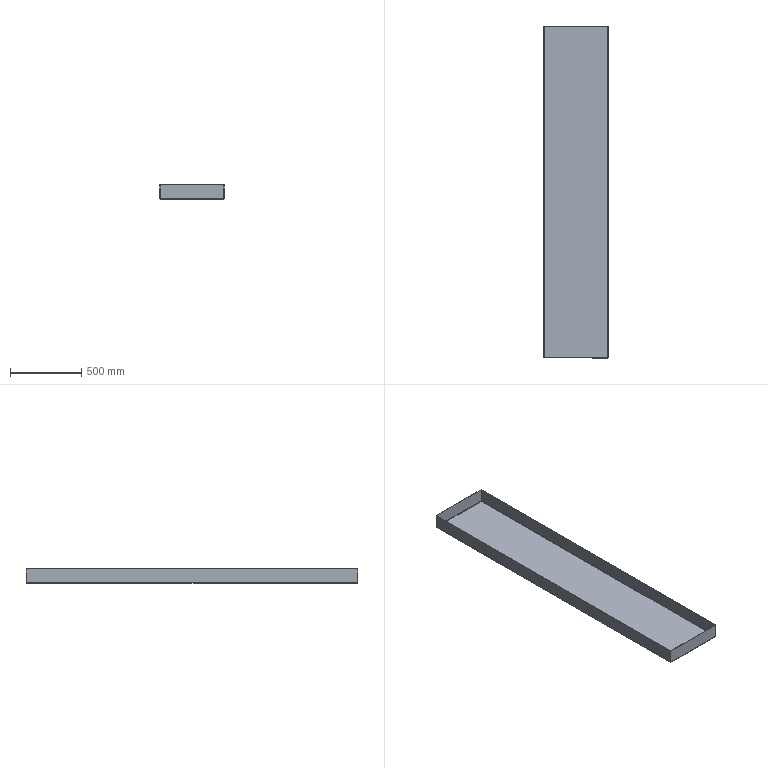Part | STEP file | 750038433 | 1 solid | 38 faces | box 450 x 2327 x 100 mm | volume 3164012 mm3 | plane 30 | cylinder 8 | commonest cylinder face diameters 4 x4 8 x4
STEP:
#1=CARTESIAN_POINT('',(-221.,2318.5,0.));
#2=VERTEX_POINT('',#1);
#3=CARTESIAN_POINT('',(221.,2318.5,0.));
#4=VERTEX_POINT('',#3);
#5=CARTESIAN_POINT('',(0.,2318.5,0.));
#6=DIRECTION('',(1.,0.,0.));
#7=VECTOR('',#6,1000.);
#8=LINE('',#5,#7);
#9=EDGE_CURVE('',#2,#4,#8,.T.);
#10=ORIENTED_EDGE('',*,*,#9,.T.);
#11=CARTESIAN_POINT('',(221.,0.,0.));
#12=VERTEX_POINT('',#11);
#13=CARTESIAN_POINT('',(221.,0.,0.));
#14=DIRECTION('',(0.,-1.,0.));
#15=VECTOR('',#14,1000.);
#16=LINE('',#13,#15);
#17=EDGE_CURVE('',#4,#12,#16,.T.);
#18=ORIENTED_EDGE('',*,*,#17,.T.);
#19=CARTESIAN_POINT('',(-221.,0.,0.));
#20=VERTEX_POINT('',#19);
#21=CARTESIAN_POINT('',(0.,0.,0.));
#22=DIRECTION('',(-1.,0.,0.));
#23=VECTOR('',#22,1000.);
#24=LINE('',#21,#23);
#25=EDGE_CURVE('',#12,#20,#24,.T.);
#26=ORIENTED_EDGE('',*,*,#25,.T.);
#27=CARTESIAN_POINT('',(-221.,0.,0.));
#28=DIRECTION('',(0.,1.,0.));
#29=VECTOR('',#28,1000.);
#30=LINE('',#27,#29);
#31=EDGE_CURVE('',#20,#2,#30,.T.);
#32=ORIENTED_EDGE('',*,*,#31,.T.);
#33=EDGE_LOOP('',(#10,#18,#26,#32));
#34=FACE_OUTER_BOUND('',#33,.T.);
#35=CARTESIAN_POINT('',(0.,0.,0.));
#36=DIRECTION('',(0.,0.,-1.));
#37=DIRECTION('',(-1.,0.,0.));
#38=AXIS2_PLACEMENT_3D('',#35,#36,#37);
#39=PLANE('',#38);
#40=ADVANCED_FACE('',(#34),#39,.T.);
#41=CARTESIAN_POINT('',(223.,2320.,0.5359));
#42=VERTEX_POINT('',#41);
#43=CARTESIAN_POINT('',(225.,2320.,4.));
#44=VERTEX_POINT('',#43);
#45=CARTESIAN_POINT('',(221.,2320.,4.));
#46=DIRECTION('',(0.,-1.,0.));
#47=DIRECTION('',(0.,0.,1.));
#48=AXIS2_PLACEMENT_3D('',#45,#46,#47);
#49=CIRCLE('',#48,4.);
#50=EDGE_CURVE('',#42,#44,#49,.T.);
#51=ORIENTED_EDGE('',*,*,#50,.T.);
#52=CARTESIAN_POINT('',(225.,-1.5,4.));
#53=VERTEX_POINT('',#52);
#54=CARTESIAN_POINT('',(225.,0.,4.));
#55=DIRECTION('',(0.,-1.,0.));
#56=VECTOR('',#55,1000.);
#57=LINE('',#54,#56);
#58=EDGE_CURVE('',#44,#53,#57,.T.);
#59=ORIENTED_EDGE('',*,*,#58,.T.);
#60=CARTESIAN_POINT('',(223.,-1.5,0.5359));
#61=VERTEX_POINT('',#60);
#62=CARTESIAN_POINT('',(221.,-1.5,4.));
#63=DIRECTION('',(0.,1.,0.));
#64=DIRECTION('',(0.,0.,1.));
#65=AXIS2_PLACEMENT_3D('',#62,#63,#64);
#66=CIRCLE('',#65,4.);
#67=EDGE_CURVE('',#53,#61,#66,.T.);
#68=ORIENTED_EDGE('',*,*,#67,.T.);
#69=CARTESIAN_POINT('',(223.,-1.5,0.5359));
#70=CARTESIAN_POINT('',(222.388,-1.041,0.1828));
#71=CARTESIAN_POINT('',(221.706,-0.5297,0.));
#72=CARTESIAN_POINT('',(221.,0.,0.));
#73=(BOUNDED_CURVE()B_SPLINE_CURVE(3,(#69,#70,#71,#72),.UNSPECIFIED.,.F.,.T.)B_SPLINE_CURVE_WITH_KNOTS((4,4),(4.189,4.712),.UNSPECIFIED.)CURVE()GEOMETRIC_REPRESENTATION_ITEM()RATIONAL_B_SPLINE_CURVE((1.,0.9773,0.9773,1.))REPRESENTATION_ITEM(''));
#74=EDGE_CURVE('',#61,#12,#73,.T.);
#75=ORIENTED_EDGE('',*,*,#74,.T.);
#76=ORIENTED_EDGE('',*,*,#17,.F.);
#77=CARTESIAN_POINT('',(221.,2318.5,0.));
#78=CARTESIAN_POINT('',(221.706,2319.03,0.));
#79=CARTESIAN_POINT('',(222.388,2319.541,0.1828));
#80=CARTESIAN_POINT('',(223.,2320.,0.5359));
#81=(BOUNDED_CURVE()B_SPLINE_CURVE(3,(#77,#78,#79,#80),.UNSPECIFIED.,.F.,.F.)B_SPLINE_CURVE_WITH_KNOTS((4,4),(4.712,5.236),.UNSPECIFIED.)CURVE()GEOMETRIC_REPRESENTATION_ITEM()RATIONAL_B_SPLINE_CURVE((1.,0.9773,0.9773,1.))REPRESENTATION_ITEM(''));
#82=EDGE_CURVE('',#4,#42,#81,.T.);
#83=ORIENTED_EDGE('',*,*,#82,.T.);
#84=EDGE_LOOP('',(#51,#59,#68,#75,#76,#83));
#85=FACE_OUTER_BOUND('',#84,.T.);
#86=CARTESIAN_POINT('',(221.,0.,4.));
#87=DIRECTION('',(0.,1.,0.));
#88=DIRECTION('',(0.,0.,1.));
#89=AXIS2_PLACEMENT_3D('',#86,#87,#88);
#90=CYLINDRICAL_SURFACE('',#89,4.);
#91=ADVANCED_FACE('',(#85),#90,.T.);
#92=CARTESIAN_POINT('',(222.5,2320.5,0.5359));
#93=VERTEX_POINT('',#92);
#94=CARTESIAN_POINT('',(222.5,2320.5,0.5359));
#95=CARTESIAN_POINT('',(222.041,2319.888,0.1828));
#96=CARTESIAN_POINT('',(221.53,2319.206,0.));
#97=CARTESIAN_POINT('',(221.,2318.5,0.));
#98=(BOUNDED_CURVE()B_SPLINE_CURVE(3,(#94,#95,#96,#97),.UNSPECIFIED.,.F.,.F.)B_SPLINE_CURVE_WITH_KNOTS((4,4),(4.189,4.712),.UNSPECIFIED.)CURVE()GEOMETRIC_REPRESENTATION_ITEM()RATIONAL_B_SPLINE_CURVE((1.,0.9773,0.9773,1.))REPRESENTATION_ITEM(''));
#99=EDGE_CURVE('',#93,#4,#98,.T.);
#100=ORIENTED_EDGE('',*,*,#99,.T.);
#101=ORIENTED_EDGE('',*,*,#9,.F.);
#102=CARTESIAN_POINT('',(-222.5,2320.5,0.5359));
#103=VERTEX_POINT('',#102);
#104=CARTESIAN_POINT('',(-221.,2318.5,0.));
#105=CARTESIAN_POINT('',(-221.53,2319.206,0.));
#106=CARTESIAN_POINT('',(-222.041,2319.888,0.1828));
#107=CARTESIAN_POINT('',(-222.5,2320.5,0.5359));
#108=(BOUNDED_CURVE()B_SPLINE_CURVE(3,(#104,#105,#106,#107),.UNSPECIFIED.,.F.,.T.)B_SPLINE_CURVE_WITH_KNOTS((4,4),(4.712,5.236),.UNSPECIFIED.)CURVE()GEOMETRIC_REPRESENTATION_ITEM()RATIONAL_B_SPLINE_CURVE((1.,0.9773,0.9773,1.))REPRESENTATION_ITEM(''));
#109=EDGE_CURVE('',#2,#103,#108,.T.);
#110=ORIENTED_EDGE('',*,*,#109,.T.);
#111=CARTESIAN_POINT('',(-222.5,2322.5,4.));
#112=VERTEX_POINT('',#111);
#113=CARTESIAN_POINT('',(-222.5,2318.5,4.));
#114=DIRECTION('',(1.,0.,0.));
#115=DIRECTION('',(0.,-1.,0.));
#116=AXIS2_PLACEMENT_3D('',#113,#114,#115);
#117=CIRCLE('',#116,4.);
#118=EDGE_CURVE('',#103,#112,#117,.T.);
#119=ORIENTED_EDGE('',*,*,#118,.T.);
#120=CARTESIAN_POINT('',(222.5,2322.5,4.));
#121=VERTEX_POINT('',#120);
#122=CARTESIAN_POINT('',(221.,2322.5,4.));
#123=DIRECTION('',(1.,0.,0.));
#124=VECTOR('',#123,1000.);
#125=LINE('',#122,#124);
#126=EDGE_CURVE('',#112,#121,#125,.T.);
#127=ORIENTED_EDGE('',*,*,#126,.T.);
#128=CARTESIAN_POINT('',(222.5,2318.5,4.));
#129=DIRECTION('',(-1.,0.,0.));
#130=DIRECTION('',(0.,-1.,0.));
#131=AXIS2_PLACEMENT_3D('',#128,#129,#130);
#132=CIRCLE('',#131,4.);
#133=EDGE_CURVE('',#121,#93,#132,.T.);
#134=ORIENTED_EDGE('',*,*,#133,.T.);
#135=EDGE_LOOP('',(#100,#101,#110,#119,#127,#134));
#136=FACE_OUTER_BOUND('',#135,.T.);
#137=CARTESIAN_POINT('',(221.,2318.5,4.));
#138=DIRECTION('',(-1.,0.,0.));
#139=DIRECTION('',(0.,-1.,0.));
#140=AXIS2_PLACEMENT_3D('',#137,#138,#139);
#141=CYLINDRICAL_SURFACE('',#140,4.);
#142=ADVANCED_FACE('',(#136),#141,.T.);
#143=CARTESIAN_POINT('',(-223.,2320.,0.5359));
#144=VERTEX_POINT('',#143);
#145=CARTESIAN_POINT('',(-223.,2320.,0.5359));
#146=CARTESIAN_POINT('',(-222.388,2319.541,0.1828));
#147=CARTESIAN_POINT('',(-221.706,2319.03,0.));
#148=CARTESIAN_POINT('',(-221.,2318.5,0.));
#149=(BOUNDED_CURVE()B_SPLINE_CURVE(3,(#145,#146,#147,#148),.UNSPECIFIED.,.F.,.F.)B_SPLINE_CURVE_WITH_KNOTS((4,4),(4.189,4.712),.UNSPECIFIED.)CURVE()GEOMETRIC_REPRESENTATION_ITEM()RATIONAL_B_SPLINE_CURVE((1.,0.9773,0.9773,1.))REPRESENTATION_ITEM(''));
#150=EDGE_CURVE('',#144,#2,#149,.T.);
#151=ORIENTED_EDGE('',*,*,#150,.T.);
#152=ORIENTED_EDGE('',*,*,#31,.F.);
#153=CARTESIAN_POINT('',(-223.,-1.5,0.5359));
#154=VERTEX_POINT('',#153);
#155=CARTESIAN_POINT('',(-221.,0.,0.));
#156=CARTESIAN_POINT('',(-221.706,-0.5297,0.));
#157=CARTESIAN_POINT('',(-222.388,-1.041,0.1828));
#158=CARTESIAN_POINT('',(-223.,-1.5,0.5359));
#159=(BOUNDED_CURVE()B_SPLINE_CURVE(3,(#155,#156,#157,#158),.UNSPECIFIED.,.F.,.T.)B_SPLINE_CURVE_WITH_KNOTS((4,4),(4.712,5.236),.UNSPECIFIED.)CURVE()GEOMETRIC_REPRESENTATION_ITEM()RATIONAL_B_SPLINE_CURVE((1.,0.9773,0.9773,1.))REPRESENTATION_ITEM(''));
#160=EDGE_CURVE('',#20,#154,#159,.T.);
#161=ORIENTED_EDGE('',*,*,#160,.T.);
#162=CARTESIAN_POINT('',(-225.,-1.5,4.));
#163=VERTEX_POINT('',#162);
#164=CARTESIAN_POINT('',(-221.,-1.5,4.));
#165=DIRECTION('',(0.,1.,0.));
#166=DIRECTION('',(0.,0.,-1.));
#167=AXIS2_PLACEMENT_3D('',#164,#165,#166);
#168=CIRCLE('',#167,4.);
#169=EDGE_CURVE('',#154,#163,#168,.T.);
#170=ORIENTED_EDGE('',*,*,#169,.T.);
#171=CARTESIAN_POINT('',(-225.,2320.,4.));
#172=VERTEX_POINT('',#171);
#173=CARTESIAN_POINT('',(-225.,2318.5,4.));
#174=DIRECTION('',(0.,1.,0.));
#175=VECTOR('',#174,1000.);
#176=LINE('',#173,#175);
#177=EDGE_CURVE('',#163,#172,#176,.T.);
#178=ORIENTED_EDGE('',*,*,#177,.T.);
#179=CARTESIAN_POINT('',(-221.,2320.,4.));
#180=DIRECTION('',(0.,-1.,0.));
#181=DIRECTION('',(0.,0.,-1.));
#182=AXIS2_PLACEMENT_3D('',#179,#180,#181);
#183=CIRCLE('',#182,4.);
#184=EDGE_CURVE('',#172,#144,#183,.T.);
#185=ORIENTED_EDGE('',*,*,#184,.T.);
#186=EDGE_LOOP('',(#151,#152,#161,#170,#178,#185));
#187=FACE_OUTER_BOUND('',#186,.T.);
#188=CARTESIAN_POINT('',(-221.,2318.5,4.));
#189=DIRECTION('',(0.,-1.,0.));
#190=DIRECTION('',(0.,0.,-1.));
#191=AXIS2_PLACEMENT_3D('',#188,#189,#190);
#192=CYLINDRICAL_SURFACE('',#191,4.);
#193=ADVANCED_FACE('',(#187),#192,.T.);
#194=CARTESIAN_POINT('',(-222.5,-2.,0.5359));
#195=VERTEX_POINT('',#194);
#196=CARTESIAN_POINT('',(-222.5,-2.,0.5359));
#197=CARTESIAN_POINT('',(-222.041,-1.388,0.1828));
#198=CARTESIAN_POINT('',(-221.53,-0.7062,0.));
#199=CARTESIAN_POINT('',(-221.,0.,0.));
#200=(BOUNDED_CURVE()B_SPLINE_CURVE(3,(#196,#197,#198,#199),.UNSPECIFIED.,.F.,.F.)B_SPLINE_CURVE_WITH_KNOTS((4,4),(4.189,4.712),.UNSPECIFIED.)CURVE()GEOMETRIC_REPRESENTATION_ITEM()RATIONAL_B_SPLINE_CURVE((1.,0.9773,0.9773,1.))REPRESENTATION_ITEM(''));
#201=EDGE_CURVE('',#195,#20,#200,.T.);
#202=ORIENTED_EDGE('',*,*,#201,.T.);
#203=ORIENTED_EDGE('',*,*,#25,.F.);
#204=CARTESIAN_POINT('',(222.5,-2.,0.5359));
#205=VERTEX_POINT('',#204);
#206=CARTESIAN_POINT('',(221.,0.,0.));
#207=CARTESIAN_POINT('',(221.53,-0.7062,0.));
#208=CARTESIAN_POINT('',(222.041,-1.388,0.1828));
#209=CARTESIAN_POINT('',(222.5,-2.,0.5359));
#210=(BOUNDED_CURVE()B_SPLINE_CURVE(3,(#206,#207,#208,#209),.UNSPECIFIED.,.F.,.F.)B_SPLINE_CURVE_WITH_KNOTS((4,4),(4.712,5.236),.UNSPECIFIED.)CURVE()GEOMETRIC_REPRESENTATION_ITEM()RATIONAL_B_SPLINE_CURVE((1.,0.9773,0.9773,1.))REPRESENTATION_ITEM(''));
#211=EDGE_CURVE('',#12,#205,#210,.T.);
#212=ORIENTED_EDGE('',*,*,#211,.T.);
#213=CARTESIAN_POINT('',(222.5,-4.,4.));
#214=VERTEX_POINT('',#213);
#215=CARTESIAN_POINT('',(222.5,0.,4.));
#216=DIRECTION('',(-1.,0.,0.));
#217=DIRECTION('',(0.,1.,0.));
#218=AXIS2_PLACEMENT_3D('',#215,#216,#217);
#219=CIRCLE('',#218,4.);
#220=EDGE_CURVE('',#205,#214,#219,.T.);
#221=ORIENTED_EDGE('',*,*,#220,.T.);
#222=CARTESIAN_POINT('',(-222.5,-4.,4.));
#223=VERTEX_POINT('',#222);
#224=CARTESIAN_POINT('',(-221.,-4.,4.));
#225=DIRECTION('',(-1.,0.,0.));
#226=VECTOR('',#225,1000.);
#227=LINE('',#224,#226);
#228=EDGE_CURVE('',#214,#223,#227,.T.);
#229=ORIENTED_EDGE('',*,*,#228,.T.);
#230=CARTESIAN_POINT('',(-222.5,0.,4.));
#231=DIRECTION('',(1.,0.,0.));
#232=DIRECTION('',(0.,1.,0.));
#233=AXIS2_PLACEMENT_3D('',#230,#231,#232);
#234=CIRCLE('',#233,4.);
#235=EDGE_CURVE('',#223,#195,#234,.T.);
#236=ORIENTED_EDGE('',*,*,#235,.T.);
#237=EDGE_LOOP('',(#202,#203,#212,#221,#229,#236));
#238=FACE_OUTER_BOUND('',#237,.T.);
#239=CARTESIAN_POINT('',(-221.,0.,4.));
#240=DIRECTION('',(1.,0.,0.));
#241=DIRECTION('',(0.,1.,0.));
#242=AXIS2_PLACEMENT_3D('',#239,#240,#241);
#243=CYLINDRICAL_SURFACE('',#242,4.);
#244=ADVANCED_FACE('',(#238),#243,.T.);
#245=CARTESIAN_POINT('',(225.,2320.,100.));
#246=VERTEX_POINT('',#245);
#247=CARTESIAN_POINT('',(225.,2320.,0.));
#248=DIRECTION('',(0.,0.,-1.));
#249=VECTOR('',#248,1000.);
#250=LINE('',#247,#249);
#251=EDGE_CURVE('',#246,#44,#250,.T.);
#252=ORIENTED_EDGE('',*,*,#251,.F.);
#253=CARTESIAN_POINT('',(225.,-1.5,100.));
#254=VERTEX_POINT('',#253);
#255=CARTESIAN_POINT('',(225.,0.,100.));
#256=DIRECTION('',(0.,1.,0.));
#257=VECTOR('',#256,1000.);
#258=LINE('',#255,#257);
#259=EDGE_CURVE('',#254,#246,#258,.T.);
#260=ORIENTED_EDGE('',*,*,#259,.F.);
#261=CARTESIAN_POINT('',(225.,-1.5,0.));
#262=DIRECTION('',(0.,0.,1.));
#263=VECTOR('',#262,1000.);
#264=LINE('',#261,#263);
#265=EDGE_CURVE('',#53,#254,#264,.T.);
#266=ORIENTED_EDGE('',*,*,#265,.F.);
#267=ORIENTED_EDGE('',*,*,#58,.F.);
#268=EDGE_LOOP('',(#252,#260,#266,#267));
#269=FACE_OUTER_BOUND('',#268,.T.);
#270=CARTESIAN_POINT('',(225.,0.,0.));
#271=DIRECTION('',(-1.,0.,0.));
#272=DIRECTION('',(0.,-1.,0.));
#273=AXIS2_PLACEMENT_3D('',#270,#271,#272);
#274=PLANE('',#273);
#275=ADVANCED_FACE('',(#269),#274,.F.);
#276=CARTESIAN_POINT('',(223.,2320.,4.));
#277=VERTEX_POINT('',#276);
#278=CARTESIAN_POINT('',(223.,2320.,100.));
#279=VERTEX_POINT('',#278);
#280=CARTESIAN_POINT('',(223.,2320.,2.));
#281=DIRECTION('',(0.,0.,1.));
#282=VECTOR('',#281,1000.);
#283=LINE('',#280,#282);
#284=EDGE_CURVE('',#277,#279,#283,.T.);
#285=ORIENTED_EDGE('',*,*,#284,.T.);
#286=CARTESIAN_POINT('',(-221.,2320.,100.));
#287=DIRECTION('',(1.,0.,0.));
#288=VECTOR('',#287,1000.);
#289=LINE('',#286,#288);
#290=EDGE_CURVE('',#279,#246,#289,.T.);
#291=ORIENTED_EDGE('',*,*,#290,.T.);
#292=ORIENTED_EDGE('',*,*,#251,.T.);
#293=ORIENTED_EDGE('',*,*,#50,.F.);
#294=CARTESIAN_POINT('',(223.,2320.,2.));
#295=DIRECTION('',(0.,0.,1.));
#296=VECTOR('',#295,1000.);
#297=LINE('',#294,#296);
#298=EDGE_CURVE('',#42,#277,#297,.T.);
#299=ORIENTED_EDGE('',*,*,#298,.T.);
#300=EDGE_LOOP('',(#285,#291,#292,#293,#299));
#301=FACE_OUTER_BOUND('',#300,.T.);
#302=CARTESIAN_POINT('',(-221.,2320.,2.));
#303=DIRECTION('',(0.,1.,0.));
#304=DIRECTION('',(0.,0.,1.));
#305=AXIS2_PLACEMENT_3D('',#302,#303,#304);
#306=PLANE('',#305);
#307=ADVANCED_FACE('',(#301),#306,.T.);
#308=ORIENTED_EDGE('',*,*,#298,.F.);
#309=ORIENTED_EDGE('',*,*,#82,.F.);
#310=CARTESIAN_POINT('',(221.,2318.5,2.));
#311=VERTEX_POINT('',#310);
#312=CARTESIAN_POINT('',(221.,2318.5,-1000.));
#313=DIRECTION('',(0.,0.,-1.));
#314=VECTOR('',#313,1000.);
#315=LINE('',#312,#314);
#316=EDGE_CURVE('',#311,#4,#315,.T.);
#317=ORIENTED_EDGE('',*,*,#316,.F.);
#318=CARTESIAN_POINT('',(223.,2320.,4.));
#319=CARTESIAN_POINT('',(223.,2320.,2.828));
#320=CARTESIAN_POINT('',(222.172,2319.379,2.));
#321=CARTESIAN_POINT('',(221.,2318.5,2.));
#322=(BOUNDED_CURVE()B_SPLINE_CURVE(3,(#318,#319,#320,#321),.UNSPECIFIED.,.F.,.F.)B_SPLINE_CURVE_WITH_KNOTS((4,4),(0.,1.571),.UNSPECIFIED.)CURVE()GEOMETRIC_REPRESENTATION_ITEM()RATIONAL_B_SPLINE_CURVE((1.,0.8047,0.8047,1.))REPRESENTATION_ITEM(''));
#323=EDGE_CURVE('',#277,#311,#322,.T.);
#324=ORIENTED_EDGE('',*,*,#323,.F.);
#325=EDGE_LOOP('',(#308,#309,#317,#324));
#326=FACE_OUTER_BOUND('',#325,.T.);
#327=CARTESIAN_POINT('',(-579.,1718.5,-1000.));
#328=DIRECTION('',(0.6,-0.8,0.));
#329=DIRECTION('',(0.8,0.6,0.));
#330=AXIS2_PLACEMENT_3D('',#327,#328,#329);
#331=PLANE('',#330);
#332=ADVANCED_FACE('',(#326),#331,.F.);
#333=CARTESIAN_POINT('',(221.,0.,2.));
#334=VERTEX_POINT('',#333);
#335=CARTESIAN_POINT('',(221.,0.,-1000.));
#336=DIRECTION('',(0.,0.,-1.));
#337=VECTOR('',#336,1000.);
#338=LINE('',#335,#337);
#339=EDGE_CURVE('',#334,#12,#338,.T.);
#340=ORIENTED_EDGE('',*,*,#339,.T.);
#341=ORIENTED_EDGE('',*,*,#74,.F.);
#342=CARTESIAN_POINT('',(223.,-1.5,4.));
#343=VERTEX_POINT('',#342);
#344=CARTESIAN_POINT('',(223.,-1.5,-1000.));
#345=DIRECTION('',(0.,0.,1.));
#346=VECTOR('',#345,1000.);
#347=LINE('',#344,#346);
#348=EDGE_CURVE('',#61,#343,#347,.T.);
#349=ORIENTED_EDGE('',*,*,#348,.T.);
#350=CARTESIAN_POINT('',(223.,-1.5,4.));
#351=CARTESIAN_POINT('',(223.,-1.5,2.828));
#352=CARTESIAN_POINT('',(222.172,-0.8787,2.));
#353=CARTESIAN_POINT('',(221.,0.,2.));
#354=(BOUNDED_CURVE()B_SPLINE_CURVE(3,(#350,#351,#352,#353),.UNSPECIFIED.,.F.,.F.)B_SPLINE_CURVE_WITH_KNOTS((4,4),(3.142,4.712),.UNSPECIFIED.)CURVE()GEOMETRIC_REPRESENTATION_ITEM()RATIONAL_B_SPLINE_CURVE((1.,0.8047,0.8047,1.))REPRESENTATION_ITEM(''));
#355=EDGE_CURVE('',#343,#334,#354,.T.);
#356=ORIENTED_EDGE('',*,*,#355,.T.);
#357=EDGE_LOOP('',(#340,#341,#349,#356));
#358=FACE_OUTER_BOUND('',#357,.T.);
#359=CARTESIAN_POINT('',(-579.,600.,-1000.));
#360=DIRECTION('',(-0.6,-0.8,0.));
#361=DIRECTION('',(0.8,-0.6,0.));
#362=AXIS2_PLACEMENT_3D('',#359,#360,#361);
#363=PLANE('',#362);
#364=ADVANCED_FACE('',(#358),#363,.T.);
#365=ORIENTED_EDGE('',*,*,#265,.T.);
#366=CARTESIAN_POINT('',(223.,-1.5,100.));
#367=VERTEX_POINT('',#366);
#368=CARTESIAN_POINT('',(221.,-1.5,100.));
#369=DIRECTION('',(-1.,0.,0.));
#370=VECTOR('',#369,1000.);
#371=LINE('',#368,#370);
#372=EDGE_CURVE('',#254,#367,#371,.T.);
#373=ORIENTED_EDGE('',*,*,#372,.T.);
#374=CARTESIAN_POINT('',(223.,-1.5,2.));
#375=DIRECTION('',(0.,0.,-1.));
#376=VECTOR('',#375,1000.);
#377=LINE('',#374,#376);
#378=EDGE_CURVE('',#367,#343,#377,.T.);
#379=ORIENTED_EDGE('',*,*,#378,.T.);
#380=ORIENTED_EDGE('',*,*,#348,.F.);
#381=ORIENTED_EDGE('',*,*,#67,.F.);
#382=EDGE_LOOP('',(#365,#373,#379,#380,#381));
#383=FACE_OUTER_BOUND('',#382,.T.);
#384=CARTESIAN_POINT('',(221.,-1.5,2.));
#385=DIRECTION('',(0.,-1.,0.));
#386=DIRECTION('',(0.,0.,-1.));
#387=AXIS2_PLACEMENT_3D('',#384,#385,#386);
#388=PLANE('',#387);
#389=ADVANCED_FACE('',(#383),#388,.T.);
#390=CARTESIAN_POINT('',(222.5,2320.5,4.));
#391=VERTEX_POINT('',#390);
#392=CARTESIAN_POINT('',(222.5,2320.5,4.));
#393=CARTESIAN_POINT('',(222.5,2320.5,2.828));
#394=CARTESIAN_POINT('',(221.879,2319.672,2.));
#395=CARTESIAN_POINT('',(221.,2318.5,2.));
#396=(BOUNDED_CURVE()B_SPLINE_CURVE(3,(#392,#393,#394,#395),.UNSPECIFIED.,.F.,.F.)B_SPLINE_CURVE_WITH_KNOTS((4,4),(3.142,4.712),.UNSPECIFIED.)CURVE()GEOMETRIC_REPRESENTATION_ITEM()RATIONAL_B_SPLINE_CURVE((1.,0.8047,0.8047,1.))REPRESENTATION_ITEM(''));
#397=EDGE_CURVE('',#391,#311,#396,.T.);
#398=ORIENTED_EDGE('',*,*,#397,.T.);
#399=ORIENTED_EDGE('',*,*,#316,.T.);
#400=ORIENTED_EDGE('',*,*,#99,.F.);
#401=CARTESIAN_POINT('',(222.5,2320.5,-1000.));
#402=DIRECTION('',(0.,0.,1.));
#403=VECTOR('',#402,1000.);
#404=LINE('',#401,#403);
#405=EDGE_CURVE('',#93,#391,#404,.T.);
#406=ORIENTED_EDGE('',*,*,#405,.T.);
#407=EDGE_LOOP('',(#398,#399,#400,#406));
#408=FACE_OUTER_BOUND('',#407,.T.);
#409=CARTESIAN_POINT('',(-379.,1518.5,-1000.));
#410=DIRECTION('',(0.8,-0.6,0.));
#411=DIRECTION('',(0.6,0.8,0.));
#412=AXIS2_PLACEMENT_3D('',#409,#410,#411);
#413=PLANE('',#412);
#414=ADVANCED_FACE('',(#408),#413,.T.);
#415=ORIENTED_EDGE('',*,*,#405,.F.);
#416=ORIENTED_EDGE('',*,*,#133,.F.);
#417=CARTESIAN_POINT('',(222.5,2322.5,100.));
#418=VERTEX_POINT('',#417);
#419=CARTESIAN_POINT('',(222.5,2322.5,100.));
#420=DIRECTION('',(0.,0.,-1.));
#421=VECTOR('',#420,1000.);
#422=LINE('',#419,#421);
#423=EDGE_CURVE('',#418,#121,#422,.T.);
#424=ORIENTED_EDGE('',*,*,#423,.F.);
#425=CARTESIAN_POINT('',(222.5,2320.5,100.));
#426=VERTEX_POINT('',#425);
#427=CARTESIAN_POINT('',(222.5,2322.5,100.));
#428=DIRECTION('',(0.,1.,0.));
#429=VECTOR('',#428,1000.);
#430=LINE('',#427,#429);
#431=EDGE_CURVE('',#426,#418,#430,.T.);
#432=ORIENTED_EDGE('',*,*,#431,.F.);
#433=CARTESIAN_POINT('',(222.5,2320.5,100.));
#434=DIRECTION('',(0.,0.,1.));
#435=VECTOR('',#434,1000.);
#436=LINE('',#433,#435);
#437=EDGE_CURVE('',#391,#426,#436,.T.);
#438=ORIENTED_EDGE('',*,*,#437,.F.);
#439=EDGE_LOOP('',(#415,#416,#424,#432,#438));
#440=FACE_OUTER_BOUND('',#439,.T.);
#441=CARTESIAN_POINT('',(222.5,2322.5,100.));
#442=DIRECTION('',(-1.,0.,0.));
#443=DIRECTION('',(0.,0.,1.));
#444=AXIS2_PLACEMENT_3D('',#441,#442,#443);
#445=PLANE('',#444);
#446=ADVANCED_FACE('',(#440),#445,.F.);
#447=CARTESIAN_POINT('',(-222.5,2322.5,100.));
#448=VERTEX_POINT('',#447);
#449=CARTESIAN_POINT('',(-222.5,2322.5,0.));
#450=DIRECTION('',(0.,0.,1.));
#451=VECTOR('',#450,1000.);
#452=LINE('',#449,#451);
#453=EDGE_CURVE('',#112,#448,#452,.T.);
#454=ORIENTED_EDGE('',*,*,#453,.T.);
#455=CARTESIAN_POINT('',(0.,2322.5,100.));
#456=DIRECTION('',(1.,0.,0.));
#457=VECTOR('',#456,1000.);
#458=LINE('',#455,#457);
#459=EDGE_CURVE('',#448,#418,#458,.T.);
#460=ORIENTED_EDGE('',*,*,#459,.T.);
#461=ORIENTED_EDGE('',*,*,#423,.T.);
#462=ORIENTED_EDGE('',*,*,#126,.F.);
#463=EDGE_LOOP('',(#454,#460,#461,#462));
#464=FACE_OUTER_BOUND('',#463,.T.);
#465=CARTESIAN_POINT('',(0.,2322.5,0.));
#466=DIRECTION('',(0.,1.,0.));
#467=DIRECTION('',(0.,0.,1.));
#468=AXIS2_PLACEMENT_3D('',#465,#466,#467);
#469=PLANE('',#468);
#470=ADVANCED_FACE('',(#464),#469,.T.);
#471=ORIENTED_EDGE('',*,*,#118,.F.);
#472=CARTESIAN_POINT('',(-222.5,2320.5,4.));
#473=VERTEX_POINT('',#472);
#474=CARTESIAN_POINT('',(-222.5,2320.5,1.911));
#475=DIRECTION('',(0.,0.,-1.));
#476=VECTOR('',#475,1000.);
#477=LINE('',#474,#476);
#478=EDGE_CURVE('',#473,#103,#477,.T.);
#479=ORIENTED_EDGE('',*,*,#478,.F.);
#480=CARTESIAN_POINT('',(-222.5,2320.5,100.));
#481=VERTEX_POINT('',#480);
#482=CARTESIAN_POINT('',(-222.5,2320.5,1.911));
#483=DIRECTION('',(0.,0.,-1.));
#484=VECTOR('',#483,1000.);
#485=LINE('',#482,#484);
#486=EDGE_CURVE('',#481,#473,#485,.T.);
#487=ORIENTED_EDGE('',*,*,#486,.F.);
#488=CARTESIAN_POINT('',(-222.5,2322.5,100.));
#489=DIRECTION('',(0.,-1.,0.));
#490=VECTOR('',#489,1000.);
#491=LINE('',#488,#490);
#492=EDGE_CURVE('',#448,#481,#491,.T.);
#493=ORIENTED_EDGE('',*,*,#492,.F.);
#494=ORIENTED_EDGE('',*,*,#453,.F.);
#495=EDGE_LOOP('',(#471,#479,#487,#493,#494));
#496=FACE_OUTER_BOUND('',#495,.T.);
#497=CARTESIAN_POINT('',(-222.5,2322.5,1.911));
#498=DIRECTION('',(1.,0.,0.));
#499=DIRECTION('',(0.,0.,-1.));
#500=AXIS2_PLACEMENT_3D('',#497,#498,#499);
#501=PLANE('',#500);
#502=ADVANCED_FACE('',(#496),#501,.F.);
#503=ORIENTED_EDGE('',*,*,#478,.T.);
#504=ORIENTED_EDGE('',*,*,#109,.F.);
#505=CARTESIAN_POINT('',(-221.,2318.5,2.));
#506=VERTEX_POINT('',#505);
#507=CARTESIAN_POINT('',(-221.,2318.5,-1000.));
#508=DIRECTION('',(0.,0.,-1.));
#509=VECTOR('',#508,1000.);
#510=LINE('',#507,#509);
#511=EDGE_CURVE('',#506,#2,#510,.T.);
#512=ORIENTED_EDGE('',*,*,#511,.F.);
#513=CARTESIAN_POINT('',(-222.5,2320.5,4.));
#514=CARTESIAN_POINT('',(-222.5,2320.5,2.828));
#515=CARTESIAN_POINT('',(-221.879,2319.672,2.));
#516=CARTESIAN_POINT('',(-221.,2318.5,2.));
#517=(BOUNDED_CURVE()B_SPLINE_CURVE(3,(#513,#514,#515,#516),.UNSPECIFIED.,.F.,.F.)B_SPLINE_CURVE_WITH_KNOTS((4,4),(0.,1.571),.UNSPECIFIED.)CURVE()GEOMETRIC_REPRESENTATION_ITEM()RATIONAL_B_SPLINE_CURVE((1.,0.8047,0.8047,1.))REPRESENTATION_ITEM(''));
#518=EDGE_CURVE('',#473,#506,#517,.T.);
#519=ORIENTED_EDGE('',*,*,#518,.F.);
#520=EDGE_LOOP('',(#503,#504,#512,#519));
#521=FACE_OUTER_BOUND('',#520,.T.);
#522=CARTESIAN_POINT('',(379.,1518.5,-1000.));
#523=DIRECTION('',(0.8,0.6,0.));
#524=DIRECTION('',(-0.6,0.8,0.));
#525=AXIS2_PLACEMENT_3D('',#522,#523,#524);
#526=PLANE('',#525);
#527=ADVANCED_FACE('',(#521),#526,.F.);
#528=CARTESIAN_POINT('',(-223.,2320.,4.));
#529=VERTEX_POINT('',#528);
#530=CARTESIAN_POINT('',(-223.,2320.,4.));
#531=CARTESIAN_POINT('',(-223.,2320.,2.828));
#532=CARTESIAN_POINT('',(-222.172,2319.379,2.));
#533=CARTESIAN_POINT('',(-221.,2318.5,2.));
#534=(BOUNDED_CURVE()B_SPLINE_CURVE(3,(#530,#531,#532,#533),.UNSPECIFIED.,.F.,.F.)B_SPLINE_CURVE_WITH_KNOTS((4,4),(3.142,4.712),.UNSPECIFIED.)CURVE()GEOMETRIC_REPRESENTATION_ITEM()RATIONAL_B_SPLINE_CURVE((1.,0.8047,0.8047,1.))REPRESENTATION_ITEM(''));
#535=EDGE_CURVE('',#529,#506,#534,.T.);
#536=ORIENTED_EDGE('',*,*,#535,.T.);
#537=ORIENTED_EDGE('',*,*,#511,.T.);
#538=ORIENTED_EDGE('',*,*,#150,.F.);
#539=CARTESIAN_POINT('',(-223.,2320.,-1000.));
#540=DIRECTION('',(0.,0.,1.));
#541=VECTOR('',#540,1000.);
#542=LINE('',#539,#541);
#543=EDGE_CURVE('',#144,#529,#542,.T.);
#544=ORIENTED_EDGE('',*,*,#543,.T.);
#545=EDGE_LOOP('',(#536,#537,#538,#544));
#546=FACE_OUTER_BOUND('',#545,.T.);
#547=CARTESIAN_POINT('',(579.,1718.5,-1000.));
#548=DIRECTION('',(0.6,0.8,0.));
#549=DIRECTION('',(-0.8,0.6,0.));
#550=AXIS2_PLACEMENT_3D('',#547,#548,#549);
#551=PLANE('',#550);
#552=ADVANCED_FACE('',(#546),#551,.T.);
#553=CARTESIAN_POINT('',(-225.,2320.,100.));
#554=VERTEX_POINT('',#553);
#555=CARTESIAN_POINT('',(-225.,2320.,2.));
#556=DIRECTION('',(0.,0.,1.));
#557=VECTOR('',#556,1000.);
#558=LINE('',#555,#557);
#559=EDGE_CURVE('',#172,#554,#558,.T.);
#560=ORIENTED_EDGE('',*,*,#559,.T.);
#561=CARTESIAN_POINT('',(-223.,2320.,100.));
#562=VERTEX_POINT('',#561);
#563=CARTESIAN_POINT('',(-221.,2320.,100.));
#564=DIRECTION('',(1.,0.,0.));
#565=VECTOR('',#564,1000.);
#566=LINE('',#563,#565);
#567=EDGE_CURVE('',#554,#562,#566,.T.);
#568=ORIENTED_EDGE('',*,*,#567,.T.);
#569=CARTESIAN_POINT('',(-223.,2320.,2.));
#570=DIRECTION('',(0.,0.,-1.));
#571=VECTOR('',#570,1000.);
#572=LINE('',#569,#571);
#573=EDGE_CURVE('',#562,#529,#572,.T.);
#574=ORIENTED_EDGE('',*,*,#573,.T.);
#575=ORIENTED_EDGE('',*,*,#543,.F.);
#576=ORIENTED_EDGE('',*,*,#184,.F.);
#577=EDGE_LOOP('',(#560,#568,#574,#575,#576));
#578=FACE_OUTER_BOUND('',#577,.T.);
#579=CARTESIAN_POINT('',(-221.,2320.,2.));
#580=DIRECTION('',(0.,1.,0.));
#581=DIRECTION('',(0.,0.,1.));
#582=AXIS2_PLACEMENT_3D('',#579,#580,#581);
#583=PLANE('',#582);
#584=ADVANCED_FACE('',(#578),#583,.T.);
#585=CARTESIAN_POINT('',(-225.,-1.5,100.));
#586=VERTEX_POINT('',#585);
#587=CARTESIAN_POINT('',(-225.,-1.5,0.));
#588=DIRECTION('',(0.,0.,1.));
#589=VECTOR('',#588,1000.);
#590=LINE('',#587,#589);
#591=EDGE_CURVE('',#163,#586,#590,.T.);
#592=ORIENTED_EDGE('',*,*,#591,.T.);
#593=CARTESIAN_POINT('',(-225.,0.,100.));
#594=DIRECTION('',(0.,1.,0.));
#595=VECTOR('',#594,1000.);
#596=LINE('',#593,#595);
#597=EDGE_CURVE('',#586,#554,#596,.T.);
#598=ORIENTED_EDGE('',*,*,#597,.T.);
#599=ORIENTED_EDGE('',*,*,#559,.F.);
#600=ORIENTED_EDGE('',*,*,#177,.F.);
#601=EDGE_LOOP('',(#592,#598,#599,#600));
#602=FACE_OUTER_BOUND('',#601,.T.);
#603=CARTESIAN_POINT('',(-225.,0.,0.));
#604=DIRECTION('',(-1.,0.,0.));
#605=DIRECTION('',(0.,-1.,0.));
#606=AXIS2_PLACEMENT_3D('',#603,#604,#605);
#607=PLANE('',#606);
#608=ADVANCED_FACE('',(#602),#607,.T.);
#609=CARTESIAN_POINT('',(-223.,-1.5,4.));
#610=VERTEX_POINT('',#609);
#611=CARTESIAN_POINT('',(-223.,-1.5,100.));
#612=VERTEX_POINT('',#611);
#613=CARTESIAN_POINT('',(-223.,-1.5,2.));
#614=DIRECTION('',(0.,0.,1.));
#615=VECTOR('',#614,1000.);
#616=LINE('',#613,#615);
#617=EDGE_CURVE('',#610,#612,#616,.T.);
#618=ORIENTED_EDGE('',*,*,#617,.T.);
#619=CARTESIAN_POINT('',(221.,-1.5,100.));
#620=DIRECTION('',(-1.,0.,0.));
#621=VECTOR('',#620,1000.);
#622=LINE('',#619,#621);
#623=EDGE_CURVE('',#612,#586,#622,.T.);
#624=ORIENTED_EDGE('',*,*,#623,.T.);
#625=ORIENTED_EDGE('',*,*,#591,.F.);
#626=ORIENTED_EDGE('',*,*,#169,.F.);
#627=CARTESIAN_POINT('',(-223.,-1.5,2.));
#628=DIRECTION('',(0.,0.,1.));
#629=VECTOR('',#628,1000.);
#630=LINE('',#627,#629);
#631=EDGE_CURVE('',#154,#610,#630,.T.);
#632=ORIENTED_EDGE('',*,*,#631,.T.);
#633=EDGE_LOOP('',(#618,#624,#625,#626,#632));
#634=FACE_OUTER_BOUND('',#633,.T.);
#635=CARTESIAN_POINT('',(221.,-1.5,2.));
#636=DIRECTION('',(0.,-1.,0.));
#637=DIRECTION('',(0.,0.,-1.));
#638=AXIS2_PLACEMENT_3D('',#635,#636,#637);
#639=PLANE('',#638);
#640=ADVANCED_FACE('',(#634),#639,.T.);
#641=ORIENTED_EDGE('',*,*,#631,.F.);
#642=ORIENTED_EDGE('',*,*,#160,.F.);
#643=CARTESIAN_POINT('',(-221.,0.,2.));
#644=VERTEX_POINT('',#643);
#645=CARTESIAN_POINT('',(-221.,0.,-1000.));
#646=DIRECTION('',(0.,0.,-1.));
#647=VECTOR('',#646,1000.);
#648=LINE('',#645,#647);
#649=EDGE_CURVE('',#644,#20,#648,.T.);
#650=ORIENTED_EDGE('',*,*,#649,.F.);
#651=CARTESIAN_POINT('',(-223.,-1.5,4.));
#652=CARTESIAN_POINT('',(-223.,-1.5,2.828));
#653=CARTESIAN_POINT('',(-222.172,-0.8787,2.));
#654=CARTESIAN_POINT('',(-221.,0.,2.));
#655=(BOUNDED_CURVE()B_SPLINE_CURVE(3,(#651,#652,#653,#654),.UNSPECIFIED.,.F.,.F.)B_SPLINE_CURVE_WITH_KNOTS((4,4),(0.,1.571),.UNSPECIFIED.)CURVE()GEOMETRIC_REPRESENTATION_ITEM()RATIONAL_B_SPLINE_CURVE((1.,0.8047,0.8047,1.))REPRESENTATION_ITEM(''));
#656=EDGE_CURVE('',#610,#644,#655,.T.);
#657=ORIENTED_EDGE('',*,*,#656,.F.);
#658=EDGE_LOOP('',(#641,#642,#650,#657));
#659=FACE_OUTER_BOUND('',#658,.T.);
#660=CARTESIAN_POINT('',(579.,600.,-1000.));
#661=DIRECTION('',(-0.6,0.8,0.));
#662=DIRECTION('',(-0.8,-0.6,0.));
#663=AXIS2_PLACEMENT_3D('',#660,#661,#662);
#664=PLANE('',#663);
#665=ADVANCED_FACE('',(#659),#664,.F.);
#666=CARTESIAN_POINT('',(-222.5,-2.,4.));
#667=VERTEX_POINT('',#666);
#668=CARTESIAN_POINT('',(-222.5,-2.,4.));
#669=CARTESIAN_POINT('',(-222.5,-2.,2.828));
#670=CARTESIAN_POINT('',(-221.879,-1.172,2.));
#671=CARTESIAN_POINT('',(-221.,0.,2.));
#672=(BOUNDED_CURVE()B_SPLINE_CURVE(3,(#668,#669,#670,#671),.UNSPECIFIED.,.F.,.F.)B_SPLINE_CURVE_WITH_KNOTS((4,4),(3.142,4.712),.UNSPECIFIED.)CURVE()GEOMETRIC_REPRESENTATION_ITEM()RATIONAL_B_SPLINE_CURVE((1.,0.8047,0.8047,1.))REPRESENTATION_ITEM(''));
#673=EDGE_CURVE('',#667,#644,#672,.T.);
#674=ORIENTED_EDGE('',*,*,#673,.T.);
#675=ORIENTED_EDGE('',*,*,#649,.T.);
#676=ORIENTED_EDGE('',*,*,#201,.F.);
#677=CARTESIAN_POINT('',(-222.5,-2.,-1000.));
#678=DIRECTION('',(0.,0.,1.));
#679=VECTOR('',#678,1000.);
#680=LINE('',#677,#679);
#681=EDGE_CURVE('',#195,#667,#680,.T.);
#682=ORIENTED_EDGE('',*,*,#681,.T.);
#683=EDGE_LOOP('',(#674,#675,#676,#682));
#684=FACE_OUTER_BOUND('',#683,.T.);
#685=CARTESIAN_POINT('',(379.,800.,-1000.));
#686=DIRECTION('',(-0.8,0.6,0.));
#687=DIRECTION('',(-0.6,-0.8,0.));
#688=AXIS2_PLACEMENT_3D('',#685,#686,#687);
#689=PLANE('',#688);
#690=ADVANCED_FACE('',(#684),#689,.T.);
#691=CARTESIAN_POINT('',(-222.5,-4.,100.));
#692=VERTEX_POINT('',#691);
#693=CARTESIAN_POINT('',(-222.5,-4.,1.911));
#694=DIRECTION('',(0.,0.,1.));
#695=VECTOR('',#694,1000.);
#696=LINE('',#693,#695);
#697=EDGE_CURVE('',#223,#692,#696,.T.);
#698=ORIENTED_EDGE('',*,*,#697,.T.);
#699=CARTESIAN_POINT('',(-222.5,-2.,100.));
#700=VERTEX_POINT('',#699);
#701=CARTESIAN_POINT('',(-222.5,-4.,100.));
#702=DIRECTION('',(0.,1.,0.));
#703=VECTOR('',#702,1000.);
#704=LINE('',#701,#703);
#705=EDGE_CURVE('',#692,#700,#704,.T.);
#706=ORIENTED_EDGE('',*,*,#705,.T.);
#707=CARTESIAN_POINT('',(-222.5,-2.,1.911));
#708=DIRECTION('',(0.,0.,-1.));
#709=VECTOR('',#708,1000.);
#710=LINE('',#707,#709);
#711=EDGE_CURVE('',#700,#667,#710,.T.);
#712=ORIENTED_EDGE('',*,*,#711,.T.);
#713=ORIENTED_EDGE('',*,*,#681,.F.);
#714=ORIENTED_EDGE('',*,*,#235,.F.);
#715=EDGE_LOOP('',(#698,#706,#712,#713,#714));
#716=FACE_OUTER_BOUND('',#715,.T.);
#717=CARTESIAN_POINT('',(-222.5,-4.,1.911));
#718=DIRECTION('',(-1.,0.,0.));
#719=DIRECTION('',(0.,-1.,0.));
#720=AXIS2_PLACEMENT_3D('',#717,#718,#719);
#721=PLANE('',#720);
#722=ADVANCED_FACE('',(#716),#721,.T.);
#723=CARTESIAN_POINT('',(222.5,-4.,100.));
#724=VERTEX_POINT('',#723);
#725=CARTESIAN_POINT('',(222.5,-4.,0.));
#726=DIRECTION('',(0.,0.,-1.));
#727=VECTOR('',#726,1000.);
#728=LINE('',#725,#727);
#729=EDGE_CURVE('',#724,#214,#728,.T.);
#730=ORIENTED_EDGE('',*,*,#729,.F.);
#731=CARTESIAN_POINT('',(0.,-4.,100.));
#732=DIRECTION('',(1.,0.,0.));
#733=VECTOR('',#732,1000.);
#734=LINE('',#731,#733);
#735=EDGE_CURVE('',#692,#724,#734,.T.);
#736=ORIENTED_EDGE('',*,*,#735,.F.);
#737=ORIENTED_EDGE('',*,*,#697,.F.);
#738=ORIENTED_EDGE('',*,*,#228,.F.);
#739=EDGE_LOOP('',(#730,#736,#737,#738));
#740=FACE_OUTER_BOUND('',#739,.T.);
#741=CARTESIAN_POINT('',(0.,-4.,0.));
#742=DIRECTION('',(0.,1.,0.));
#743=DIRECTION('',(-1.,0.,0.));
#744=AXIS2_PLACEMENT_3D('',#741,#742,#743);
#745=PLANE('',#744);
#746=ADVANCED_FACE('',(#740),#745,.F.);
#747=CARTESIAN_POINT('',(222.5,-2.,4.));
#748=VERTEX_POINT('',#747);
#749=CARTESIAN_POINT('',(222.5,-2.,100.));
#750=VERTEX_POINT('',#749);
#751=CARTESIAN_POINT('',(222.5,-2.,100.));
#752=DIRECTION('',(0.,0.,1.));
#753=VECTOR('',#752,1000.);
#754=LINE('',#751,#753);
#755=EDGE_CURVE('',#748,#750,#754,.T.);
#756=ORIENTED_EDGE('',*,*,#755,.T.);
#757=CARTESIAN_POINT('',(222.5,-4.,100.));
#758=DIRECTION('',(0.,-1.,0.));
#759=VECTOR('',#758,1000.);
#760=LINE('',#757,#759);
#761=EDGE_CURVE('',#750,#724,#760,.T.);
#762=ORIENTED_EDGE('',*,*,#761,.T.);
#763=ORIENTED_EDGE('',*,*,#729,.T.);
#764=ORIENTED_EDGE('',*,*,#220,.F.);
#765=CARTESIAN_POINT('',(222.5,-2.,100.));
#766=DIRECTION('',(0.,0.,1.));
#767=VECTOR('',#766,1000.);
#768=LINE('',#765,#767);
#769=EDGE_CURVE('',#205,#748,#768,.T.);
#770=ORIENTED_EDGE('',*,*,#769,.T.);
#771=EDGE_LOOP('',(#756,#762,#763,#764,#770));
#772=FACE_OUTER_BOUND('',#771,.T.);
#773=CARTESIAN_POINT('',(222.5,-4.,100.));
#774=DIRECTION('',(1.,0.,0.));
#775=DIRECTION('',(0.,1.,0.));
#776=AXIS2_PLACEMENT_3D('',#773,#774,#775);
#777=PLANE('',#776);
#778=ADVANCED_FACE('',(#772),#777,.T.);
#779=ORIENTED_EDGE('',*,*,#769,.F.);
#780=ORIENTED_EDGE('',*,*,#211,.F.);
#781=ORIENTED_EDGE('',*,*,#339,.F.);
#782=CARTESIAN_POINT('',(222.5,-2.,4.));
#783=CARTESIAN_POINT('',(222.5,-2.,2.828));
#784=CARTESIAN_POINT('',(221.879,-1.172,2.));
#785=CARTESIAN_POINT('',(221.,0.,2.));
#786=(BOUNDED_CURVE()B_SPLINE_CURVE(3,(#782,#783,#784,#785),.UNSPECIFIED.,.F.,.T.)B_SPLINE_CURVE_WITH_KNOTS((4,4),(0.,1.571),.UNSPECIFIED.)CURVE()GEOMETRIC_REPRESENTATION_ITEM()RATIONAL_B_SPLINE_CURVE((1.,0.8047,0.8047,1.))REPRESENTATION_ITEM(''));
#787=EDGE_CURVE('',#748,#334,#786,.T.);
#788=ORIENTED_EDGE('',*,*,#787,.F.);
#789=EDGE_LOOP('',(#779,#780,#781,#788));
#790=FACE_OUTER_BOUND('',#789,.T.);
#791=CARTESIAN_POINT('',(-379.,800.,-1000.));
#792=DIRECTION('',(-0.8,-0.6,0.));
#793=DIRECTION('',(0.6,-0.8,0.));
#794=AXIS2_PLACEMENT_3D('',#791,#792,#793);
#795=PLANE('',#794);
#796=ADVANCED_FACE('',(#790),#795,.F.);
#797=ORIENTED_EDGE('',*,*,#259,.T.);
#798=ORIENTED_EDGE('',*,*,#290,.F.);
#799=CARTESIAN_POINT('',(223.,0.,100.));
#800=DIRECTION('',(0.,-1.,0.));
#801=VECTOR('',#800,1000.);
#802=LINE('',#799,#801);
#803=EDGE_CURVE('',#279,#367,#802,.T.);
#804=ORIENTED_EDGE('',*,*,#803,.T.);
#805=ORIENTED_EDGE('',*,*,#372,.F.);
#806=EDGE_LOOP('',(#797,#798,#804,#805));
#807=FACE_OUTER_BOUND('',#806,.T.);
#808=CARTESIAN_POINT('',(225.,0.,100.));
#809=DIRECTION('',(0.,0.,1.));
#810=DIRECTION('',(0.,-1.,0.));
#811=AXIS2_PLACEMENT_3D('',#808,#809,#810);
#812=PLANE('',#811);
#813=ADVANCED_FACE('',(#807),#812,.T.);
#814=ORIENTED_EDGE('',*,*,#378,.F.);
#815=ORIENTED_EDGE('',*,*,#803,.F.);
#816=ORIENTED_EDGE('',*,*,#284,.F.);
#817=CARTESIAN_POINT('',(223.,0.,4.));
#818=DIRECTION('',(0.,-1.,0.));
#819=VECTOR('',#818,1000.);
#820=LINE('',#817,#819);
#821=EDGE_CURVE('',#277,#343,#820,.T.);
#822=ORIENTED_EDGE('',*,*,#821,.T.);
#823=EDGE_LOOP('',(#814,#815,#816,#822));
#824=FACE_OUTER_BOUND('',#823,.T.);
#825=CARTESIAN_POINT('',(223.,0.,0.));
#826=DIRECTION('',(-1.,0.,0.));
#827=DIRECTION('',(0.,-1.,0.));
#828=AXIS2_PLACEMENT_3D('',#825,#826,#827);
#829=PLANE('',#828);
#830=ADVANCED_FACE('',(#824),#829,.T.);
#831=ORIENTED_EDGE('',*,*,#821,.F.);
#832=ORIENTED_EDGE('',*,*,#323,.T.);
#833=CARTESIAN_POINT('',(221.,0.,2.));
#834=DIRECTION('',(0.,1.,0.));
#835=VECTOR('',#834,1000.);
#836=LINE('',#833,#835);
#837=EDGE_CURVE('',#334,#311,#836,.T.);
#838=ORIENTED_EDGE('',*,*,#837,.F.);
#839=ORIENTED_EDGE('',*,*,#355,.F.);
#840=EDGE_LOOP('',(#831,#832,#838,#839));
#841=FACE_OUTER_BOUND('',#840,.T.);
#842=CARTESIAN_POINT('',(221.,0.,4.));
#843=DIRECTION('',(0.,1.,0.));
#844=DIRECTION('',(0.,0.,1.));
#845=AXIS2_PLACEMENT_3D('',#842,#843,#844);
#846=CYLINDRICAL_SURFACE('',#845,2.);
#847=ADVANCED_FACE('',(#841),#846,.F.);
#848=ORIENTED_EDGE('',*,*,#518,.T.);
#849=CARTESIAN_POINT('',(221.,2318.5,2.));
#850=DIRECTION('',(-1.,0.,0.));
#851=VECTOR('',#850,1000.);
#852=LINE('',#849,#851);
#853=EDGE_CURVE('',#311,#506,#852,.T.);
#854=ORIENTED_EDGE('',*,*,#853,.F.);
#855=ORIENTED_EDGE('',*,*,#397,.F.);
#856=CARTESIAN_POINT('',(221.,2320.5,4.));
#857=DIRECTION('',(1.,0.,0.));
#858=VECTOR('',#857,1000.);
#859=LINE('',#856,#858);
#860=EDGE_CURVE('',#473,#391,#859,.T.);
#861=ORIENTED_EDGE('',*,*,#860,.F.);
#862=EDGE_LOOP('',(#848,#854,#855,#861));
#863=FACE_OUTER_BOUND('',#862,.T.);
#864=CARTESIAN_POINT('',(221.,2318.5,4.));
#865=DIRECTION('',(-1.,0.,0.));
#866=DIRECTION('',(0.,-1.,0.));
#867=AXIS2_PLACEMENT_3D('',#864,#865,#866);
#868=CYLINDRICAL_SURFACE('',#867,2.);
#869=ADVANCED_FACE('',(#863),#868,.F.);
#870=ORIENTED_EDGE('',*,*,#437,.T.);
#871=CARTESIAN_POINT('',(0.,2320.5,100.));
#872=DIRECTION('',(1.,0.,0.));
#873=VECTOR('',#872,1000.);
#874=LINE('',#871,#873);
#875=EDGE_CURVE('',#481,#426,#874,.T.);
#876=ORIENTED_EDGE('',*,*,#875,.F.);
#877=ORIENTED_EDGE('',*,*,#486,.T.);
#878=ORIENTED_EDGE('',*,*,#860,.T.);
#879=EDGE_LOOP('',(#870,#876,#877,#878));
#880=FACE_OUTER_BOUND('',#879,.T.);
#881=CARTESIAN_POINT('',(0.,2320.5,0.));
#882=DIRECTION('',(0.,1.,0.));
#883=DIRECTION('',(0.,0.,1.));
#884=AXIS2_PLACEMENT_3D('',#881,#882,#883);
#885=PLANE('',#884);
#886=ADVANCED_FACE('',(#880),#885,.F.);
#887=ORIENTED_EDGE('',*,*,#431,.T.);
#888=ORIENTED_EDGE('',*,*,#459,.F.);
#889=ORIENTED_EDGE('',*,*,#492,.T.);
#890=ORIENTED_EDGE('',*,*,#875,.T.);
#891=EDGE_LOOP('',(#887,#888,#889,#890));
#892=FACE_OUTER_BOUND('',#891,.T.);
#893=CARTESIAN_POINT('',(-221.,2322.5,100.));
#894=DIRECTION('',(0.,0.,-1.));
#895=DIRECTION('',(-1.,0.,0.));
#896=AXIS2_PLACEMENT_3D('',#893,#894,#895);
#897=PLANE('',#896);
#898=ADVANCED_FACE('',(#892),#897,.F.);
#899=ORIENTED_EDGE('',*,*,#656,.T.);
#900=CARTESIAN_POINT('',(-221.,2318.5,2.));
#901=DIRECTION('',(0.,-1.,0.));
#902=VECTOR('',#901,1000.);
#903=LINE('',#900,#902);
#904=EDGE_CURVE('',#506,#644,#903,.T.);
#905=ORIENTED_EDGE('',*,*,#904,.F.);
#906=ORIENTED_EDGE('',*,*,#535,.F.);
#907=CARTESIAN_POINT('',(-223.,2318.5,4.));
#908=DIRECTION('',(0.,1.,0.));
#909=VECTOR('',#908,1000.);
#910=LINE('',#907,#909);
#911=EDGE_CURVE('',#610,#529,#910,.T.);
#912=ORIENTED_EDGE('',*,*,#911,.F.);
#913=EDGE_LOOP('',(#899,#905,#906,#912));
#914=FACE_OUTER_BOUND('',#913,.T.);
#915=CARTESIAN_POINT('',(-221.,2318.5,4.));
#916=DIRECTION('',(0.,-1.,0.));
#917=DIRECTION('',(0.,0.,-1.));
#918=AXIS2_PLACEMENT_3D('',#915,#916,#917);
#919=CYLINDRICAL_SURFACE('',#918,2.);
#920=ADVANCED_FACE('',(#914),#919,.F.);
#921=ORIENTED_EDGE('',*,*,#567,.F.);
#922=ORIENTED_EDGE('',*,*,#597,.F.);
#923=ORIENTED_EDGE('',*,*,#623,.F.);
#924=CARTESIAN_POINT('',(-223.,0.,100.));
#925=DIRECTION('',(0.,-1.,0.));
#926=VECTOR('',#925,1000.);
#927=LINE('',#924,#926);
#928=EDGE_CURVE('',#562,#612,#927,.T.);
#929=ORIENTED_EDGE('',*,*,#928,.F.);
#930=EDGE_LOOP('',(#921,#922,#923,#929));
#931=FACE_OUTER_BOUND('',#930,.T.);
#932=CARTESIAN_POINT('',(-225.,0.,100.));
#933=DIRECTION('',(0.,0.,-1.));
#934=DIRECTION('',(0.,1.,0.));
#935=AXIS2_PLACEMENT_3D('',#932,#933,#934);
#936=PLANE('',#935);
#937=ADVANCED_FACE('',(#931),#936,.F.);
#938=ORIENTED_EDGE('',*,*,#573,.F.);
#939=ORIENTED_EDGE('',*,*,#928,.T.);
#940=ORIENTED_EDGE('',*,*,#617,.F.);
#941=ORIENTED_EDGE('',*,*,#911,.T.);
#942=EDGE_LOOP('',(#938,#939,#940,#941));
#943=FACE_OUTER_BOUND('',#942,.T.);
#944=CARTESIAN_POINT('',(-223.,0.,0.));
#945=DIRECTION('',(-1.,0.,0.));
#946=DIRECTION('',(0.,-1.,0.));
#947=AXIS2_PLACEMENT_3D('',#944,#945,#946);
#948=PLANE('',#947);
#949=ADVANCED_FACE('',(#943),#948,.F.);
#950=ORIENTED_EDGE('',*,*,#787,.T.);
#951=CARTESIAN_POINT('',(-221.,0.,2.));
#952=DIRECTION('',(1.,0.,0.));
#953=VECTOR('',#952,1000.);
#954=LINE('',#951,#953);
#955=EDGE_CURVE('',#644,#334,#954,.T.);
#956=ORIENTED_EDGE('',*,*,#955,.F.);
#957=ORIENTED_EDGE('',*,*,#673,.F.);
#958=CARTESIAN_POINT('',(-221.,-2.,4.));
#959=DIRECTION('',(-1.,0.,0.));
#960=VECTOR('',#959,1000.);
#961=LINE('',#958,#960);
#962=EDGE_CURVE('',#748,#667,#961,.T.);
#963=ORIENTED_EDGE('',*,*,#962,.F.);
#964=EDGE_LOOP('',(#950,#956,#957,#963));
#965=FACE_OUTER_BOUND('',#964,.T.);
#966=CARTESIAN_POINT('',(-221.,0.,4.));
#967=DIRECTION('',(1.,0.,0.));
#968=DIRECTION('',(0.,1.,0.));
#969=AXIS2_PLACEMENT_3D('',#966,#967,#968);
#970=CYLINDRICAL_SURFACE('',#969,2.);
#971=ADVANCED_FACE('',(#965),#970,.F.);
#972=ORIENTED_EDGE('',*,*,#735,.T.);
#973=ORIENTED_EDGE('',*,*,#761,.F.);
#974=CARTESIAN_POINT('',(-221.,-2.,100.));
#975=DIRECTION('',(-1.,0.,0.));
#976=VECTOR('',#975,1000.);
#977=LINE('',#974,#976);
#978=EDGE_CURVE('',#750,#700,#977,.T.);
#979=ORIENTED_EDGE('',*,*,#978,.T.);
#980=ORIENTED_EDGE('',*,*,#705,.F.);
#981=EDGE_LOOP('',(#972,#973,#979,#980));
#982=FACE_OUTER_BOUND('',#981,.T.);
#983=CARTESIAN_POINT('',(-221.,-4.,100.));
#984=DIRECTION('',(0.,0.,1.));
#985=DIRECTION('',(0.,-1.,0.));
#986=AXIS2_PLACEMENT_3D('',#983,#984,#985);
#987=PLANE('',#986);
#988=ADVANCED_FACE('',(#982),#987,.T.);
#989=ORIENTED_EDGE('',*,*,#711,.F.);
#990=ORIENTED_EDGE('',*,*,#978,.F.);
#991=ORIENTED_EDGE('',*,*,#755,.F.);
#992=ORIENTED_EDGE('',*,*,#962,.T.);
#993=EDGE_LOOP('',(#989,#990,#991,#992));
#994=FACE_OUTER_BOUND('',#993,.T.);
#995=CARTESIAN_POINT('',(0.,-2.,0.));
#996=DIRECTION('',(0.,1.,0.));
#997=DIRECTION('',(-1.,0.,0.));
#998=AXIS2_PLACEMENT_3D('',#995,#996,#997);
#999=PLANE('',#998);
#1000=ADVANCED_FACE('',(#994),#999,.T.);
#1001=ORIENTED_EDGE('',*,*,#837,.T.);
#1002=ORIENTED_EDGE('',*,*,#853,.T.);
#1003=ORIENTED_EDGE('',*,*,#904,.T.);
#1004=ORIENTED_EDGE('',*,*,#955,.T.);
#1005=EDGE_LOOP('',(#1001,#1002,#1003,#1004));
#1006=FACE_OUTER_BOUND('',#1005,.T.);
#1007=CARTESIAN_POINT('',(0.,0.,2.));
#1008=DIRECTION('',(0.,0.,-1.));
#1009=DIRECTION('',(-1.,0.,0.));
#1010=AXIS2_PLACEMENT_3D('',#1007,#1008,#1009);
#1011=PLANE('',#1010);
#1012=ADVANCED_FACE('',(#1006),#1011,.F.);
#1013=CLOSED_SHELL('',(#40,#91,#142,#193,#244,#275,#307,#332,#364,#389,#414,#446,#470,#502,#527,#552,#584,#608,#640,#665,#690,#722,#746,#778,#796,#813,#830,#847,#869,#886,#898,#920,#937,#949,#971,#988,#1000,#1012));
#1014=MANIFOLD_SOLID_BREP('',#1013);
#1015=CARTESIAN_POINT('',(0.,0.,0.));
#1016=DIRECTION('',(0.,0.,1.));
#1017=DIRECTION('',(1.,0.,0.));
#1018=AXIS2_PLACEMENT_3D('',#1015,#1016,#1017);
#1019=(LENGTH_UNIT()NAMED_UNIT(*)SI_UNIT(.MILLI.,.METRE.));
#1020=UNCERTAINTY_MEASURE_WITH_UNIT(LENGTH_MEASURE(0.00001),#1019,'','');
#1021=(NAMED_UNIT(*)PLANE_ANGLE_UNIT()SI_UNIT($,.RADIAN.));
#1022=(NAMED_UNIT(*)SI_UNIT($,.STERADIAN.)SOLID_ANGLE_UNIT());
#1023=(GEOMETRIC_REPRESENTATION_CONTEXT(3)GLOBAL_UNCERTAINTY_ASSIGNED_CONTEXT((#1020))GLOBAL_UNIT_ASSIGNED_CONTEXT((#1019,#1021,#1022))REPRESENTATION_CONTEXT('',''));
#1024=ADVANCED_BREP_SHAPE_REPRESENTATION('',(#1014,#1018),#1023);